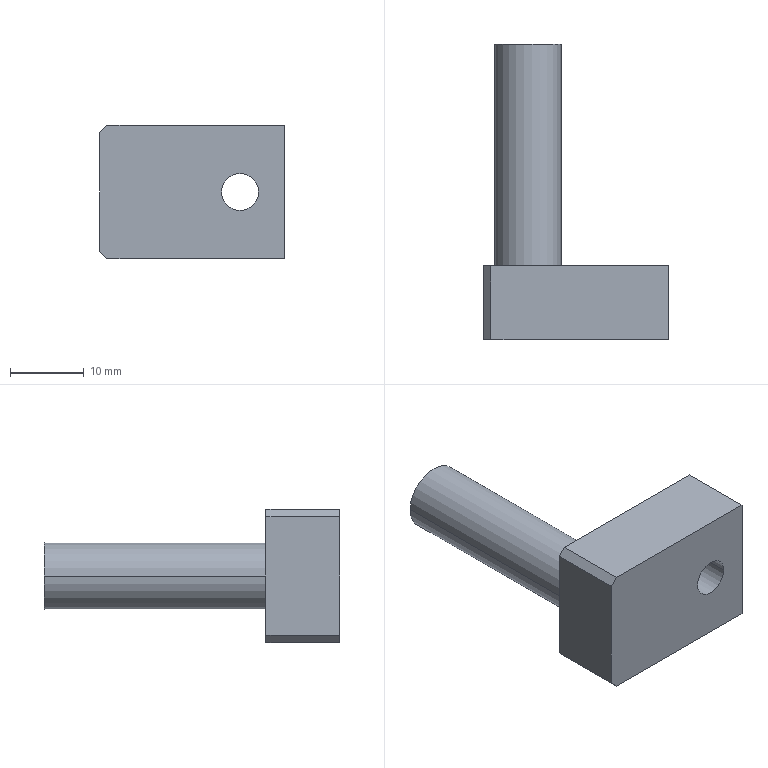Part | SolidWorks | features ICE 2, Chamfer 1, Extrusion 1 | 1 solid | 13 faces | box 25 x 40 x 18 mm | volume 6202 mm3 | plane 9 | cylinder 4 | commonest cylinder face diameters 5 x2 9 x2
STEP:
#1=CARTESIAN_POINT('',(4.,-5.,9.));
#2=VERTEX_POINT('',#1);
#3=CARTESIAN_POINT('',(9.,-5.,9.));
#4=VERTEX_POINT('',#3);
#5=CARTESIAN_POINT('',(6.5,-5.,9.));
#6=DIRECTION('',(0.,-1.,0.));
#7=DIRECTION('',(-1.,0.,0.));
#8=AXIS2_PLACEMENT_3D('',#5,#6,#7);
#9=CIRCLE('',#8,2.5);
#10=EDGE_CURVE('',#2,#4,#9,.T.);
#11=ORIENTED_EDGE('',*,*,#10,.T.);
#12=CARTESIAN_POINT('',(9.,5.,9.));
#13=VERTEX_POINT('',#12);
#14=CARTESIAN_POINT('',(9.,-5.001,9.));
#15=DIRECTION('',(0.,1.,0.));
#16=VECTOR('',#15,1000.);
#17=LINE('',#14,#16);
#18=EDGE_CURVE('',#4,#13,#17,.T.);
#19=ORIENTED_EDGE('',*,*,#18,.T.);
#20=CARTESIAN_POINT('',(4.,5.,9.));
#21=VERTEX_POINT('',#20);
#22=CARTESIAN_POINT('',(6.5,5.,9.));
#23=DIRECTION('',(0.,1.,0.));
#24=DIRECTION('',(-1.,0.,0.));
#25=AXIS2_PLACEMENT_3D('',#22,#23,#24);
#26=CIRCLE('',#25,2.5);
#27=EDGE_CURVE('',#13,#21,#26,.T.);
#28=ORIENTED_EDGE('',*,*,#27,.T.);
#29=CARTESIAN_POINT('',(4.,-5.001,9.));
#30=DIRECTION('',(0.,1.,0.));
#31=VECTOR('',#30,1000.);
#32=LINE('',#29,#31);
#33=EDGE_CURVE('',#2,#21,#32,.T.);
#34=ORIENTED_EDGE('',*,*,#33,.F.);
#35=EDGE_LOOP('',(#11,#19,#28,#34));
#36=FACE_OUTER_BOUND('',#35,.T.);
#37=CARTESIAN_POINT('',(6.5,-5.001,9.));
#38=DIRECTION('',(0.,1.,0.));
#39=DIRECTION('',(-1.,0.,0.));
#40=AXIS2_PLACEMENT_3D('',#37,#38,#39);
#41=CYLINDRICAL_SURFACE('',#40,2.5);
#42=ADVANCED_FACE('',(#36),#41,.F.);
#43=CARTESIAN_POINT('',(-11.,35.,9.));
#44=VERTEX_POINT('',#43);
#45=CARTESIAN_POINT('',(-2.,35.,9.));
#46=VERTEX_POINT('',#45);
#47=CARTESIAN_POINT('',(-6.5,35.,9.));
#48=DIRECTION('',(0.,1.,0.));
#49=DIRECTION('',(-1.,0.,0.));
#50=AXIS2_PLACEMENT_3D('',#47,#48,#49);
#51=CIRCLE('',#50,4.5);
#52=EDGE_CURVE('',#44,#46,#51,.T.);
#53=ORIENTED_EDGE('',*,*,#52,.F.);
#54=CARTESIAN_POINT('',(-11.,5.,9.));
#55=VERTEX_POINT('',#54);
#56=CARTESIAN_POINT('',(-11.,35.,9.));
#57=DIRECTION('',(0.,-1.,0.));
#58=VECTOR('',#57,1000.);
#59=LINE('',#56,#58);
#60=EDGE_CURVE('',#44,#55,#59,.T.);
#61=ORIENTED_EDGE('',*,*,#60,.T.);
#62=CARTESIAN_POINT('',(-2.,5.,9.));
#63=VERTEX_POINT('',#62);
#64=CARTESIAN_POINT('',(-6.5,5.,9.));
#65=DIRECTION('',(0.,1.,0.));
#66=DIRECTION('',(1.,0.,0.));
#67=AXIS2_PLACEMENT_3D('',#64,#65,#66);
#68=CIRCLE('',#67,4.5);
#69=EDGE_CURVE('',#55,#63,#68,.T.);
#70=ORIENTED_EDGE('',*,*,#69,.T.);
#71=CARTESIAN_POINT('',(-2.,35.,9.));
#72=DIRECTION('',(0.,-1.,0.));
#73=VECTOR('',#72,1000.);
#74=LINE('',#71,#73);
#75=EDGE_CURVE('',#46,#63,#74,.T.);
#76=ORIENTED_EDGE('',*,*,#75,.F.);
#77=EDGE_LOOP('',(#53,#61,#70,#76));
#78=FACE_OUTER_BOUND('',#77,.T.);
#79=CARTESIAN_POINT('',(-6.5,35.,9.));
#80=DIRECTION('',(0.,-1.,0.));
#81=DIRECTION('',(1.,0.,0.));
#82=AXIS2_PLACEMENT_3D('',#79,#80,#81);
#83=CYLINDRICAL_SURFACE('',#82,4.5);
#84=ADVANCED_FACE('',(#78),#83,.T.);
#85=CARTESIAN_POINT('',(-12.5,-5.,17.));
#86=VERTEX_POINT('',#85);
#87=CARTESIAN_POINT('',(-12.5,-5.,1.));
#88=VERTEX_POINT('',#87);
#89=CARTESIAN_POINT('',(-12.5,-5.,18.));
#90=DIRECTION('',(0.,0.,-1.));
#91=VECTOR('',#90,1000.);
#92=LINE('',#89,#91);
#93=EDGE_CURVE('',#86,#88,#92,.T.);
#94=ORIENTED_EDGE('',*,*,#93,.F.);
#95=CARTESIAN_POINT('',(-12.5,5.,17.));
#96=VERTEX_POINT('',#95);
#97=CARTESIAN_POINT('',(-12.5,5.,17.));
#98=DIRECTION('',(0.,1.,0.));
#99=VECTOR('',#98,1000.);
#100=LINE('',#97,#99);
#101=EDGE_CURVE('',#86,#96,#100,.T.);
#102=ORIENTED_EDGE('',*,*,#101,.T.);
#103=CARTESIAN_POINT('',(-12.5,5.,1.));
#104=VERTEX_POINT('',#103);
#105=CARTESIAN_POINT('',(-12.5,5.,18.));
#106=DIRECTION('',(0.,0.,-1.));
#107=VECTOR('',#106,1000.);
#108=LINE('',#105,#107);
#109=EDGE_CURVE('',#96,#104,#108,.T.);
#110=ORIENTED_EDGE('',*,*,#109,.T.);
#111=CARTESIAN_POINT('',(-12.5,-5.,1.));
#112=DIRECTION('',(0.,-1.,0.));
#113=VECTOR('',#112,1000.);
#114=LINE('',#111,#113);
#115=EDGE_CURVE('',#104,#88,#114,.T.);
#116=ORIENTED_EDGE('',*,*,#115,.T.);
#117=EDGE_LOOP('',(#94,#102,#110,#116));
#118=FACE_OUTER_BOUND('',#117,.T.);
#119=CARTESIAN_POINT('',(-12.5,-5.,18.));
#120=DIRECTION('',(1.,0.,0.));
#121=DIRECTION('',(0.,0.,-1.));
#122=AXIS2_PLACEMENT_3D('',#119,#120,#121);
#123=PLANE('',#122);
#124=ADVANCED_FACE('',(#118),#123,.F.);
#125=ORIENTED_EDGE('',*,*,#10,.F.);
#126=CARTESIAN_POINT('',(6.5,-5.,9.));
#127=DIRECTION('',(0.,-1.,0.));
#128=DIRECTION('',(-1.,0.,0.));
#129=AXIS2_PLACEMENT_3D('',#126,#127,#128);
#130=CIRCLE('',#129,2.5);
#131=EDGE_CURVE('',#4,#2,#130,.T.);
#132=ORIENTED_EDGE('',*,*,#131,.F.);
#133=EDGE_LOOP('',(#125,#132));
#134=FACE_BOUND('',#133,.T.);
#135=CARTESIAN_POINT('',(-11.5,-5.,18.));
#136=VERTEX_POINT('',#135);
#137=CARTESIAN_POINT('',(12.5,-5.,18.));
#138=VERTEX_POINT('',#137);
#139=CARTESIAN_POINT('',(12.5,-5.,18.));
#140=DIRECTION('',(1.,0.,0.));
#141=VECTOR('',#140,1000.);
#142=LINE('',#139,#141);
#143=EDGE_CURVE('',#136,#138,#142,.T.);
#144=ORIENTED_EDGE('',*,*,#143,.F.);
#145=CARTESIAN_POINT('',(-11.5,-5.,18.));
#146=DIRECTION('',(-0.7071,0.,-0.7071));
#147=VECTOR('',#146,1000.);
#148=LINE('',#145,#147);
#149=EDGE_CURVE('',#136,#86,#148,.T.);
#150=ORIENTED_EDGE('',*,*,#149,.T.);
#151=ORIENTED_EDGE('',*,*,#93,.T.);
#152=CARTESIAN_POINT('',(-11.5,-5.,0.));
#153=VERTEX_POINT('',#152);
#154=CARTESIAN_POINT('',(-12.5,-5.,1.));
#155=DIRECTION('',(0.7071,0.,-0.7071));
#156=VECTOR('',#155,1000.);
#157=LINE('',#154,#156);
#158=EDGE_CURVE('',#88,#153,#157,.T.);
#159=ORIENTED_EDGE('',*,*,#158,.T.);
#160=CARTESIAN_POINT('',(12.5,-5.,0.));
#161=VERTEX_POINT('',#160);
#162=CARTESIAN_POINT('',(12.5,-5.,0.));
#163=DIRECTION('',(1.,0.,0.));
#164=VECTOR('',#163,1000.);
#165=LINE('',#162,#164);
#166=EDGE_CURVE('',#153,#161,#165,.T.);
#167=ORIENTED_EDGE('',*,*,#166,.T.);
#168=CARTESIAN_POINT('',(12.5,-5.,18.));
#169=DIRECTION('',(0.,0.,-1.));
#170=VECTOR('',#169,1000.);
#171=LINE('',#168,#170);
#172=EDGE_CURVE('',#138,#161,#171,.T.);
#173=ORIENTED_EDGE('',*,*,#172,.F.);
#174=EDGE_LOOP('',(#144,#150,#151,#159,#167,#173));
#175=FACE_OUTER_BOUND('',#174,.T.);
#176=CARTESIAN_POINT('',(12.5,-5.,18.));
#177=DIRECTION('',(0.,1.,0.));
#178=DIRECTION('',(-1.,0.,0.));
#179=AXIS2_PLACEMENT_3D('',#176,#177,#178);
#180=PLANE('',#179);
#181=ADVANCED_FACE('',(#134,#175),#180,.F.);
#182=CARTESIAN_POINT('',(12.5,5.,0.));
#183=VERTEX_POINT('',#182);
#184=CARTESIAN_POINT('',(12.5,-5.,0.));
#185=DIRECTION('',(0.,1.,0.));
#186=VECTOR('',#185,1000.);
#187=LINE('',#184,#186);
#188=EDGE_CURVE('',#161,#183,#187,.T.);
#189=ORIENTED_EDGE('',*,*,#188,.T.);
#190=CARTESIAN_POINT('',(12.5,5.,18.));
#191=VERTEX_POINT('',#190);
#192=CARTESIAN_POINT('',(12.5,5.,18.));
#193=DIRECTION('',(0.,0.,-1.));
#194=VECTOR('',#193,1000.);
#195=LINE('',#192,#194);
#196=EDGE_CURVE('',#191,#183,#195,.T.);
#197=ORIENTED_EDGE('',*,*,#196,.F.);
#198=CARTESIAN_POINT('',(12.5,-5.,18.));
#199=DIRECTION('',(0.,1.,0.));
#200=VECTOR('',#199,1000.);
#201=LINE('',#198,#200);
#202=EDGE_CURVE('',#138,#191,#201,.T.);
#203=ORIENTED_EDGE('',*,*,#202,.F.);
#204=ORIENTED_EDGE('',*,*,#172,.T.);
#205=EDGE_LOOP('',(#189,#197,#203,#204));
#206=FACE_OUTER_BOUND('',#205,.T.);
#207=CARTESIAN_POINT('',(12.5,-5.,18.));
#208=DIRECTION('',(-1.,0.,0.));
#209=DIRECTION('',(0.,0.,1.));
#210=AXIS2_PLACEMENT_3D('',#207,#208,#209);
#211=PLANE('',#210);
#212=ADVANCED_FACE('',(#206),#211,.F.);
#213=CARTESIAN_POINT('',(6.5,5.,9.));
#214=DIRECTION('',(0.,1.,0.));
#215=DIRECTION('',(-1.,0.,0.));
#216=AXIS2_PLACEMENT_3D('',#213,#214,#215);
#217=CIRCLE('',#216,2.5);
#218=EDGE_CURVE('',#21,#13,#217,.T.);
#219=ORIENTED_EDGE('',*,*,#218,.F.);
#220=ORIENTED_EDGE('',*,*,#27,.F.);
#221=EDGE_LOOP('',(#219,#220));
#222=FACE_BOUND('',#221,.T.);
#223=CARTESIAN_POINT('',(-6.5,5.,9.));
#224=DIRECTION('',(0.,1.,0.));
#225=DIRECTION('',(1.,0.,0.));
#226=AXIS2_PLACEMENT_3D('',#223,#224,#225);
#227=CIRCLE('',#226,4.5);
#228=EDGE_CURVE('',#63,#55,#227,.T.);
#229=ORIENTED_EDGE('',*,*,#228,.F.);
#230=ORIENTED_EDGE('',*,*,#69,.F.);
#231=EDGE_LOOP('',(#229,#230));
#232=FACE_BOUND('',#231,.T.);
#233=ORIENTED_EDGE('',*,*,#109,.F.);
#234=CARTESIAN_POINT('',(-11.5,5.,18.));
#235=VERTEX_POINT('',#234);
#236=CARTESIAN_POINT('',(-11.5,5.,18.));
#237=DIRECTION('',(0.7071,0.,0.7071));
#238=VECTOR('',#237,1000.);
#239=LINE('',#236,#238);
#240=EDGE_CURVE('',#96,#235,#239,.T.);
#241=ORIENTED_EDGE('',*,*,#240,.T.);
#242=CARTESIAN_POINT('',(12.5,5.,18.));
#243=DIRECTION('',(-1.,0.,0.));
#244=VECTOR('',#243,1000.);
#245=LINE('',#242,#244);
#246=EDGE_CURVE('',#191,#235,#245,.T.);
#247=ORIENTED_EDGE('',*,*,#246,.F.);
#248=ORIENTED_EDGE('',*,*,#196,.T.);
#249=CARTESIAN_POINT('',(-11.5,5.,0.));
#250=VERTEX_POINT('',#249);
#251=CARTESIAN_POINT('',(12.5,5.,0.));
#252=DIRECTION('',(-1.,0.,0.));
#253=VECTOR('',#252,1000.);
#254=LINE('',#251,#253);
#255=EDGE_CURVE('',#183,#250,#254,.T.);
#256=ORIENTED_EDGE('',*,*,#255,.T.);
#257=CARTESIAN_POINT('',(-12.5,5.,1.));
#258=DIRECTION('',(-0.7071,0.,0.7071));
#259=VECTOR('',#258,1000.);
#260=LINE('',#257,#259);
#261=EDGE_CURVE('',#250,#104,#260,.T.);
#262=ORIENTED_EDGE('',*,*,#261,.T.);
#263=EDGE_LOOP('',(#233,#241,#247,#248,#256,#262));
#264=FACE_OUTER_BOUND('',#263,.T.);
#265=CARTESIAN_POINT('',(12.5,5.,18.));
#266=DIRECTION('',(0.,-1.,0.));
#267=DIRECTION('',(1.,0.,0.));
#268=AXIS2_PLACEMENT_3D('',#265,#266,#267);
#269=PLANE('',#268);
#270=ADVANCED_FACE('',(#222,#232,#264),#269,.F.);
#271=ORIENTED_EDGE('',*,*,#246,.T.);
#272=CARTESIAN_POINT('',(-11.5,-5.,18.));
#273=DIRECTION('',(0.,-1.,0.));
#274=VECTOR('',#273,1000.);
#275=LINE('',#272,#274);
#276=EDGE_CURVE('',#235,#136,#275,.T.);
#277=ORIENTED_EDGE('',*,*,#276,.T.);
#278=ORIENTED_EDGE('',*,*,#143,.T.);
#279=ORIENTED_EDGE('',*,*,#202,.T.);
#280=EDGE_LOOP('',(#271,#277,#278,#279));
#281=FACE_OUTER_BOUND('',#280,.T.);
#282=CARTESIAN_POINT('',(0.,0.,18.));
#283=DIRECTION('',(0.,0.,1.));
#284=DIRECTION('',(1.,0.,0.));
#285=AXIS2_PLACEMENT_3D('',#282,#283,#284);
#286=PLANE('',#285);
#287=ADVANCED_FACE('',(#281),#286,.T.);
#288=ORIENTED_EDGE('',*,*,#166,.F.);
#289=CARTESIAN_POINT('',(-11.5,0.,0.));
#290=DIRECTION('',(0.,1.,0.));
#291=VECTOR('',#290,1000.);
#292=LINE('',#289,#291);
#293=EDGE_CURVE('',#153,#250,#292,.T.);
#294=ORIENTED_EDGE('',*,*,#293,.T.);
#295=ORIENTED_EDGE('',*,*,#255,.F.);
#296=ORIENTED_EDGE('',*,*,#188,.F.);
#297=EDGE_LOOP('',(#288,#294,#295,#296));
#298=FACE_OUTER_BOUND('',#297,.T.);
#299=CARTESIAN_POINT('',(0.,0.,0.));
#300=DIRECTION('',(0.,0.,1.));
#301=DIRECTION('',(1.,0.,0.));
#302=AXIS2_PLACEMENT_3D('',#299,#300,#301);
#303=PLANE('',#302);
#304=ADVANCED_FACE('',(#298),#303,.F.);
#305=ORIENTED_EDGE('',*,*,#60,.F.);
#306=CARTESIAN_POINT('',(-6.5,35.,9.));
#307=DIRECTION('',(0.,1.,0.));
#308=DIRECTION('',(-1.,0.,0.));
#309=AXIS2_PLACEMENT_3D('',#306,#307,#308);
#310=CIRCLE('',#309,4.5);
#311=EDGE_CURVE('',#46,#44,#310,.T.);
#312=ORIENTED_EDGE('',*,*,#311,.F.);
#313=ORIENTED_EDGE('',*,*,#75,.T.);
#314=ORIENTED_EDGE('',*,*,#228,.T.);
#315=EDGE_LOOP('',(#305,#312,#313,#314));
#316=FACE_OUTER_BOUND('',#315,.T.);
#317=CARTESIAN_POINT('',(-6.5,35.,9.));
#318=DIRECTION('',(0.,-1.,0.));
#319=DIRECTION('',(1.,0.,0.));
#320=AXIS2_PLACEMENT_3D('',#317,#318,#319);
#321=CYLINDRICAL_SURFACE('',#320,4.5);
#322=ADVANCED_FACE('',(#316),#321,.T.);
#323=ORIENTED_EDGE('',*,*,#311,.T.);
#324=ORIENTED_EDGE('',*,*,#52,.T.);
#325=EDGE_LOOP('',(#323,#324));
#326=FACE_OUTER_BOUND('',#325,.T.);
#327=CARTESIAN_POINT('',(-6.5,35.,9.));
#328=DIRECTION('',(0.,1.,0.));
#329=DIRECTION('',(-1.,0.,0.));
#330=AXIS2_PLACEMENT_3D('',#327,#328,#329);
#331=PLANE('',#330);
#332=ADVANCED_FACE('',(#326),#331,.T.);
#333=ORIENTED_EDGE('',*,*,#18,.F.);
#334=ORIENTED_EDGE('',*,*,#131,.T.);
#335=ORIENTED_EDGE('',*,*,#33,.T.);
#336=ORIENTED_EDGE('',*,*,#218,.T.);
#337=EDGE_LOOP('',(#333,#334,#335,#336));
#338=FACE_OUTER_BOUND('',#337,.T.);
#339=CARTESIAN_POINT('',(6.5,-5.001,9.));
#340=DIRECTION('',(0.,1.,0.));
#341=DIRECTION('',(-1.,0.,0.));
#342=AXIS2_PLACEMENT_3D('',#339,#340,#341);
#343=CYLINDRICAL_SURFACE('',#342,2.5);
#344=ADVANCED_FACE('',(#338),#343,.F.);
#345=ORIENTED_EDGE('',*,*,#240,.F.);
#346=ORIENTED_EDGE('',*,*,#101,.F.);
#347=ORIENTED_EDGE('',*,*,#149,.F.);
#348=ORIENTED_EDGE('',*,*,#276,.F.);
#349=EDGE_LOOP('',(#345,#346,#347,#348));
#350=FACE_OUTER_BOUND('',#349,.T.);
#351=CARTESIAN_POINT('',(-11.5,0.,18.));
#352=DIRECTION('',(-0.7071,0.,0.7071));
#353=DIRECTION('',(0.,1.,0.));
#354=AXIS2_PLACEMENT_3D('',#351,#352,#353);
#355=PLANE('',#354);
#356=ADVANCED_FACE('',(#350),#355,.T.);
#357=ORIENTED_EDGE('',*,*,#261,.F.);
#358=ORIENTED_EDGE('',*,*,#293,.F.);
#359=ORIENTED_EDGE('',*,*,#158,.F.);
#360=ORIENTED_EDGE('',*,*,#115,.F.);
#361=EDGE_LOOP('',(#357,#358,#359,#360));
#362=FACE_OUTER_BOUND('',#361,.T.);
#363=CARTESIAN_POINT('',(-12.5,-5.,1.));
#364=DIRECTION('',(0.7071,0.,0.7071));
#365=DIRECTION('',(0.,-1.,0.));
#366=AXIS2_PLACEMENT_3D('',#363,#364,#365);
#367=PLANE('',#366);
#368=ADVANCED_FACE('',(#362),#367,.F.);
#369=CLOSED_SHELL('',(#42,#84,#124,#181,#212,#270,#287,#304,#322,#332,#344,#356,#368));
#370=MANIFOLD_SOLID_BREP('',#369);
#371=CARTESIAN_POINT('',(0.,0.,0.));
#372=DIRECTION('',(0.,0.,1.));
#373=DIRECTION('',(1.,0.,0.));
#374=AXIS2_PLACEMENT_3D('',#371,#372,#373);
#375=(LENGTH_UNIT()NAMED_UNIT(*)SI_UNIT(.MILLI.,.METRE.));
#376=UNCERTAINTY_MEASURE_WITH_UNIT(LENGTH_MEASURE(0.00001),#375,'','');
#377=(NAMED_UNIT(*)PLANE_ANGLE_UNIT()SI_UNIT($,.RADIAN.));
#378=(NAMED_UNIT(*)SI_UNIT($,.STERADIAN.)SOLID_ANGLE_UNIT());
#379=(GEOMETRIC_REPRESENTATION_CONTEXT(3)GLOBAL_UNCERTAINTY_ASSIGNED_CONTEXT((#376))GLOBAL_UNIT_ASSIGNED_CONTEXT((#375,#377,#378))REPRESENTATION_CONTEXT('',''));
#380=ADVANCED_BREP_SHAPE_REPRESENTATION('',(#370,#374),#379);